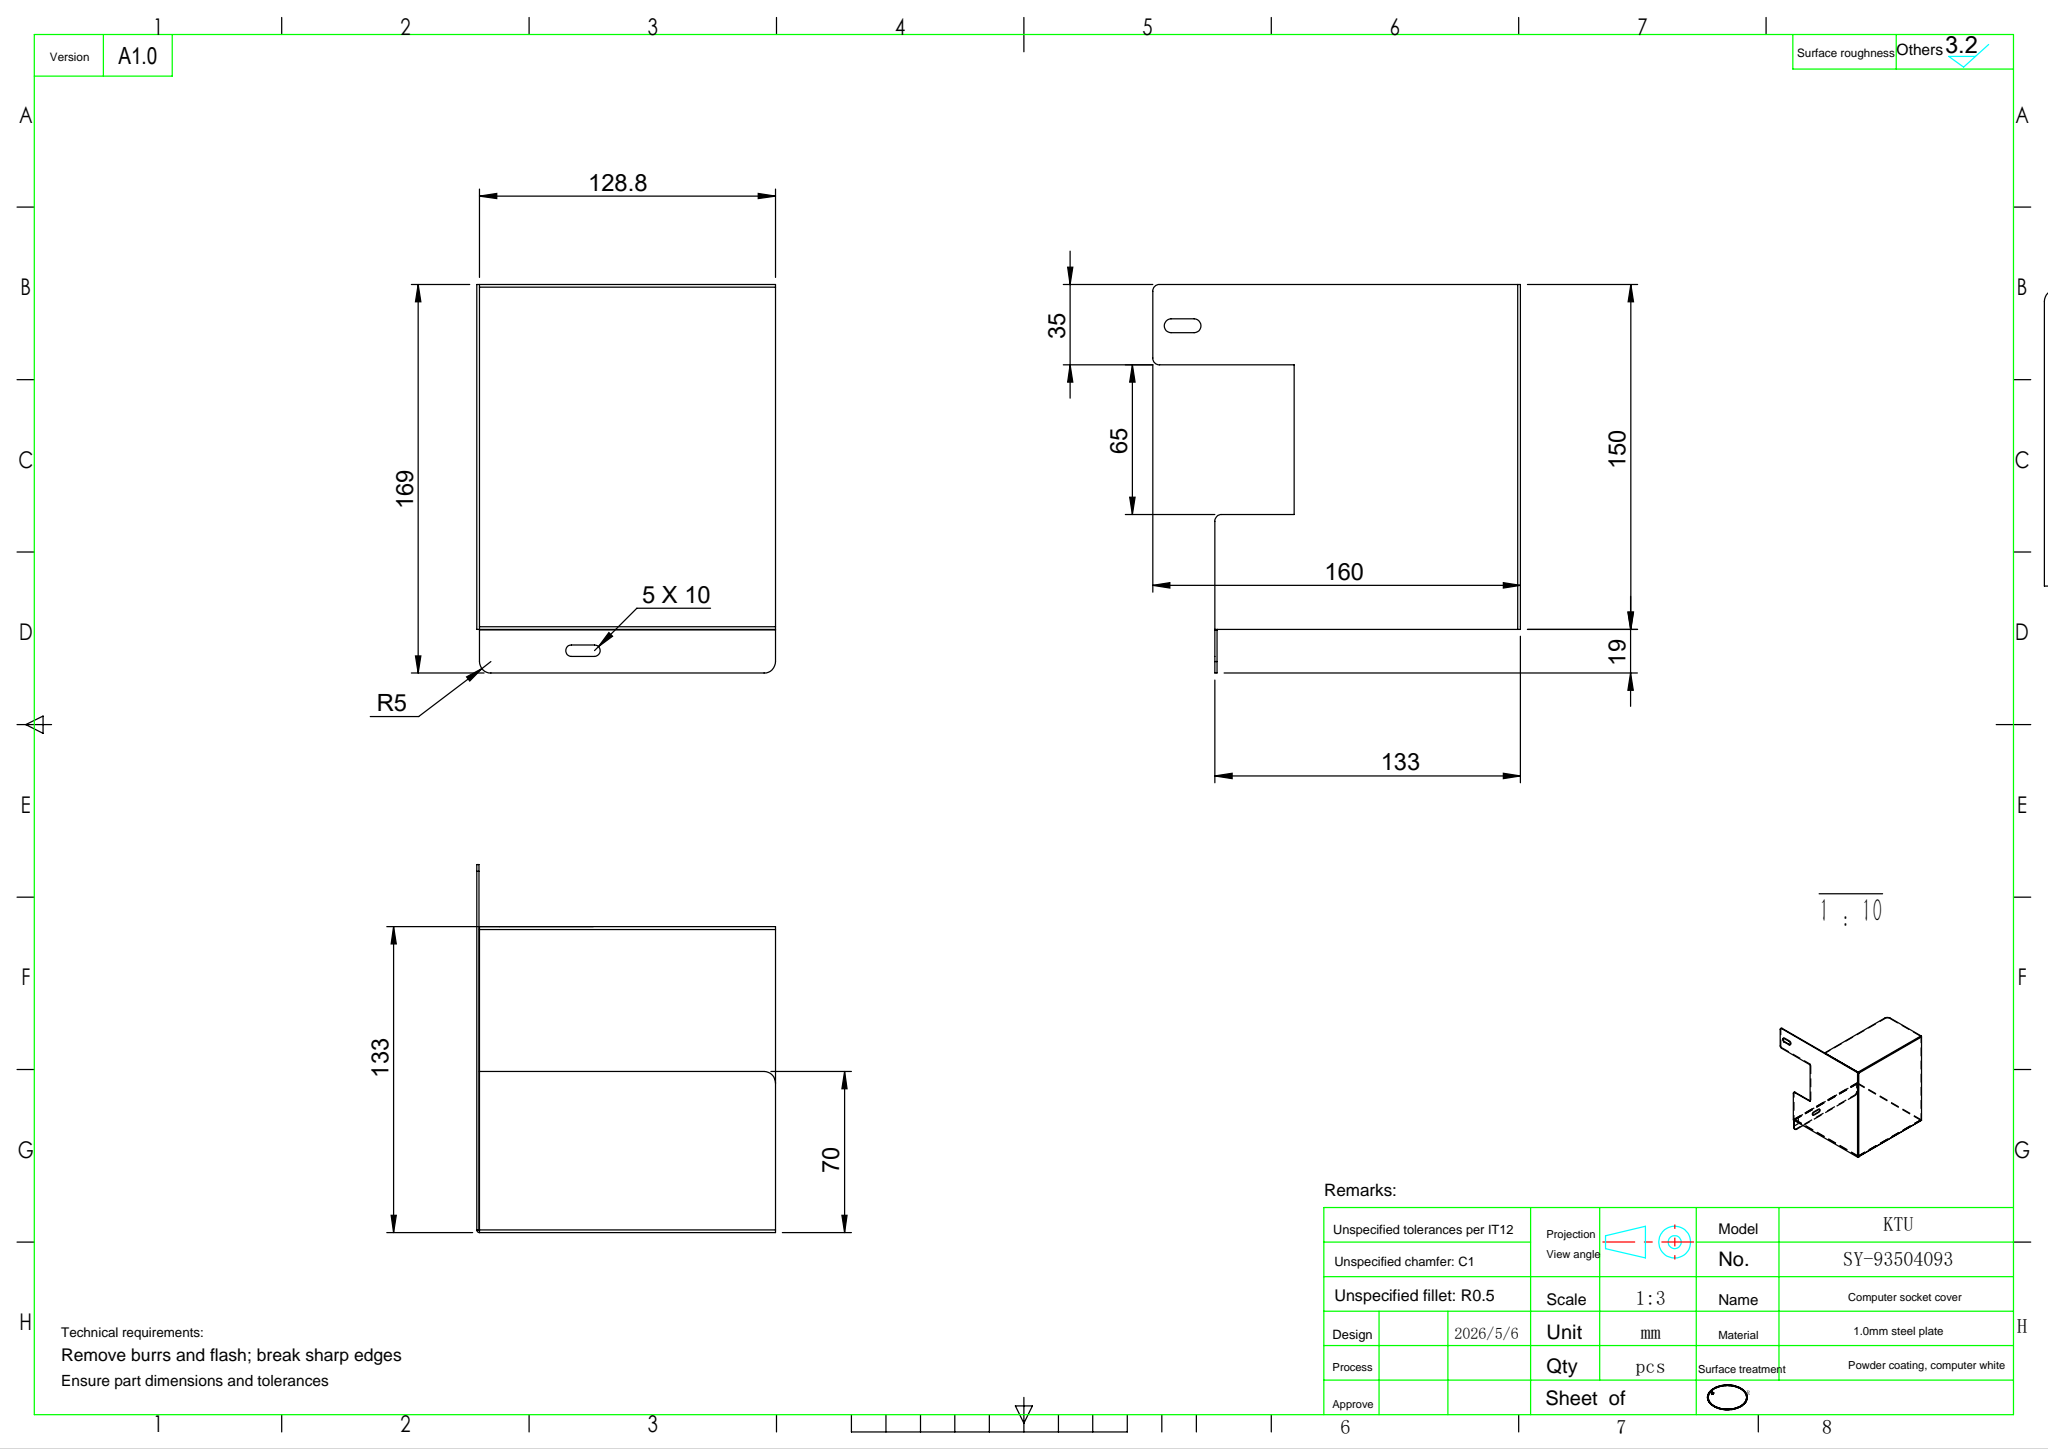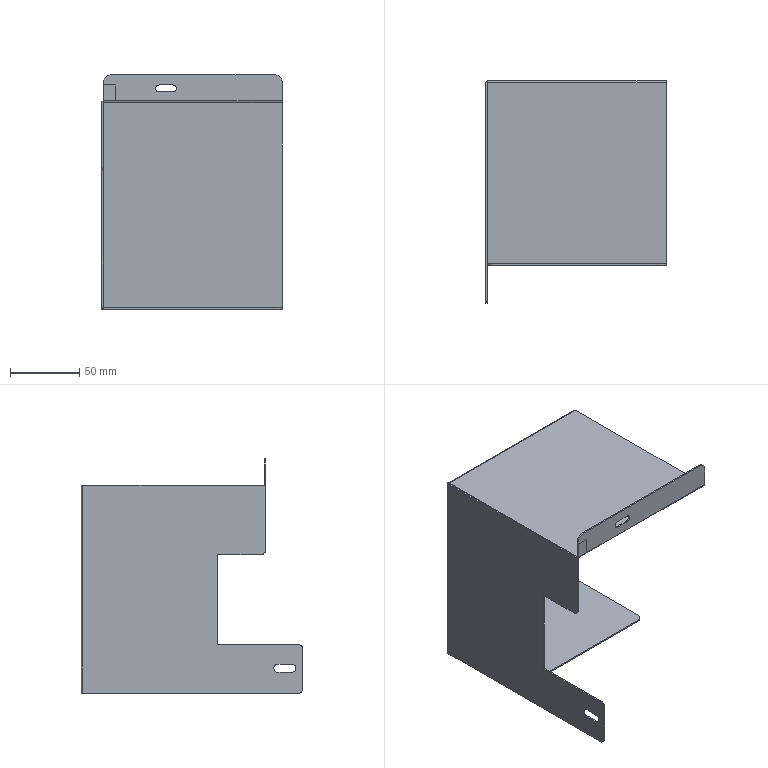Part | SolidWorks | features Fillet 4, ICE 4, EdgeFlange 3, FlatPattern 1, SMBaseFlange 1, SheetMetal 1 | 1 solid | 59 faces | box 130 x 160 x 169 mm | volume 65999 mm3 | plane 41 | cylinder 18 | commonest cylinder face diameters 6 x5 0.4 x4 2.4 x4 10 x3 5 x2